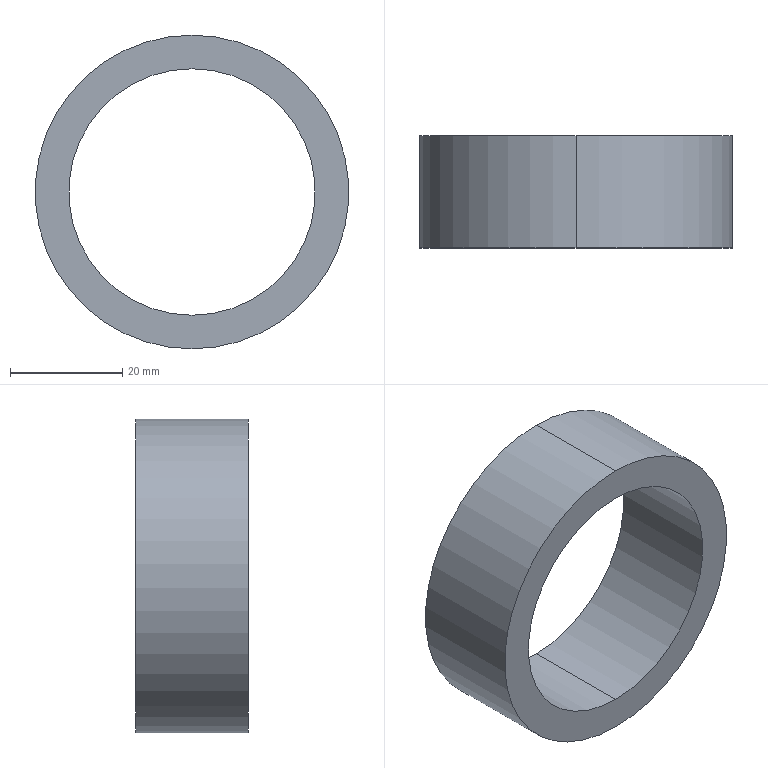Part | STEP file | outer coil2 | 1 solid | 6 faces | box 56 x 20 x 56 mm | volume 18850 mm3 | cylinder 4 | plane 2 | commonest cylinder face diameters 44 x2 56 x2
STEP:
#1=CARTESIAN_POINT('',(0.,-10.,28.));
#2=VERTEX_POINT('',#1);
#3=CARTESIAN_POINT('',(0.,-10.,-28.));
#4=VERTEX_POINT('',#3);
#5=CARTESIAN_POINT('',(0.,-10.,0.));
#6=DIRECTION('',(0.,1.,0.));
#7=DIRECTION('',(0.,0.,1.));
#8=AXIS2_PLACEMENT_3D('',#5,#6,#7);
#9=CIRCLE('',#8,28.);
#10=EDGE_CURVE('',#2,#4,#9,.T.);
#11=ORIENTED_EDGE('',*,*,#10,.T.);
#12=CARTESIAN_POINT('',(0.,10.,-28.));
#13=VERTEX_POINT('',#12);
#14=CARTESIAN_POINT('',(0.,52.348,-28.));
#15=DIRECTION('',(0.,1.,0.));
#16=VECTOR('',#15,1000.);
#17=LINE('',#14,#16);
#18=EDGE_CURVE('',#4,#13,#17,.T.);
#19=ORIENTED_EDGE('',*,*,#18,.T.);
#20=CARTESIAN_POINT('',(0.,10.,28.));
#21=VERTEX_POINT('',#20);
#22=CARTESIAN_POINT('',(0.,10.,0.));
#23=DIRECTION('',(0.,1.,0.));
#24=DIRECTION('',(0.,0.,1.));
#25=AXIS2_PLACEMENT_3D('',#22,#23,#24);
#26=CIRCLE('',#25,28.);
#27=EDGE_CURVE('',#21,#13,#26,.T.);
#28=ORIENTED_EDGE('',*,*,#27,.F.);
#29=CARTESIAN_POINT('',(0.,52.348,28.));
#30=DIRECTION('',(0.,1.,0.));
#31=VECTOR('',#30,1000.);
#32=LINE('',#29,#31);
#33=EDGE_CURVE('',#2,#21,#32,.T.);
#34=ORIENTED_EDGE('',*,*,#33,.F.);
#35=EDGE_LOOP('',(#11,#19,#28,#34));
#36=FACE_OUTER_BOUND('',#35,.T.);
#37=CARTESIAN_POINT('',(0.,52.348,0.));
#38=DIRECTION('',(0.,1.,0.));
#39=DIRECTION('',(0.,0.,1.));
#40=AXIS2_PLACEMENT_3D('',#37,#38,#39);
#41=CYLINDRICAL_SURFACE('',#40,28.);
#42=ADVANCED_FACE('',(#36),#41,.T.);
#43=CARTESIAN_POINT('',(0.,-10.,-22.));
#44=VERTEX_POINT('',#43);
#45=CARTESIAN_POINT('',(0.,-10.,22.));
#46=VERTEX_POINT('',#45);
#47=CARTESIAN_POINT('',(0.,-10.,0.));
#48=DIRECTION('',(0.,1.,0.));
#49=DIRECTION('',(0.,0.,1.));
#50=AXIS2_PLACEMENT_3D('',#47,#48,#49);
#51=CIRCLE('',#50,22.);
#52=EDGE_CURVE('',#44,#46,#51,.T.);
#53=ORIENTED_EDGE('',*,*,#52,.F.);
#54=CARTESIAN_POINT('',(0.,10.,-22.));
#55=VERTEX_POINT('',#54);
#56=CARTESIAN_POINT('',(0.,52.348,-22.));
#57=DIRECTION('',(0.,1.,0.));
#58=VECTOR('',#57,1000.);
#59=LINE('',#56,#58);
#60=EDGE_CURVE('',#44,#55,#59,.T.);
#61=ORIENTED_EDGE('',*,*,#60,.T.);
#62=CARTESIAN_POINT('',(0.,10.,22.));
#63=VERTEX_POINT('',#62);
#64=CARTESIAN_POINT('',(0.,10.,0.));
#65=DIRECTION('',(0.,1.,0.));
#66=DIRECTION('',(0.,0.,1.));
#67=AXIS2_PLACEMENT_3D('',#64,#65,#66);
#68=CIRCLE('',#67,22.);
#69=EDGE_CURVE('',#55,#63,#68,.T.);
#70=ORIENTED_EDGE('',*,*,#69,.T.);
#71=CARTESIAN_POINT('',(0.,52.348,22.));
#72=DIRECTION('',(0.,1.,0.));
#73=VECTOR('',#72,1000.);
#74=LINE('',#71,#73);
#75=EDGE_CURVE('',#46,#63,#74,.T.);
#76=ORIENTED_EDGE('',*,*,#75,.F.);
#77=EDGE_LOOP('',(#53,#61,#70,#76));
#78=FACE_OUTER_BOUND('',#77,.T.);
#79=CARTESIAN_POINT('',(0.,52.348,0.));
#80=DIRECTION('',(0.,1.,0.));
#81=DIRECTION('',(0.,0.,1.));
#82=AXIS2_PLACEMENT_3D('',#79,#80,#81);
#83=CYLINDRICAL_SURFACE('',#82,22.);
#84=ADVANCED_FACE('',(#78),#83,.F.);
#85=ORIENTED_EDGE('',*,*,#60,.F.);
#86=CARTESIAN_POINT('',(0.,-10.,0.));
#87=DIRECTION('',(0.,1.,0.));
#88=DIRECTION('',(0.,0.,1.));
#89=AXIS2_PLACEMENT_3D('',#86,#87,#88);
#90=CIRCLE('',#89,22.);
#91=EDGE_CURVE('',#46,#44,#90,.T.);
#92=ORIENTED_EDGE('',*,*,#91,.F.);
#93=ORIENTED_EDGE('',*,*,#75,.T.);
#94=CARTESIAN_POINT('',(0.,10.,0.));
#95=DIRECTION('',(0.,1.,0.));
#96=DIRECTION('',(0.,0.,1.));
#97=AXIS2_PLACEMENT_3D('',#94,#95,#96);
#98=CIRCLE('',#97,22.);
#99=EDGE_CURVE('',#63,#55,#98,.T.);
#100=ORIENTED_EDGE('',*,*,#99,.T.);
#101=EDGE_LOOP('',(#85,#92,#93,#100));
#102=FACE_OUTER_BOUND('',#101,.T.);
#103=CARTESIAN_POINT('',(0.,52.348,0.));
#104=DIRECTION('',(0.,1.,0.));
#105=DIRECTION('',(0.,0.,1.));
#106=AXIS2_PLACEMENT_3D('',#103,#104,#105);
#107=CYLINDRICAL_SURFACE('',#106,22.);
#108=ADVANCED_FACE('',(#102),#107,.F.);
#109=ORIENTED_EDGE('',*,*,#27,.T.);
#110=CARTESIAN_POINT('',(0.,10.,0.));
#111=DIRECTION('',(0.,1.,0.));
#112=DIRECTION('',(0.,0.,1.));
#113=AXIS2_PLACEMENT_3D('',#110,#111,#112);
#114=CIRCLE('',#113,28.);
#115=EDGE_CURVE('',#13,#21,#114,.T.);
#116=ORIENTED_EDGE('',*,*,#115,.T.);
#117=EDGE_LOOP('',(#109,#116));
#118=FACE_OUTER_BOUND('',#117,.T.);
#119=ORIENTED_EDGE('',*,*,#99,.F.);
#120=ORIENTED_EDGE('',*,*,#69,.F.);
#121=EDGE_LOOP('',(#119,#120));
#122=FACE_BOUND('',#121,.T.);
#123=CARTESIAN_POINT('',(-28.,10.,0.));
#124=DIRECTION('',(0.,1.,0.));
#125=DIRECTION('',(0.,0.,1.));
#126=AXIS2_PLACEMENT_3D('',#123,#124,#125);
#127=PLANE('',#126);
#128=ADVANCED_FACE('',(#118,#122),#127,.T.);
#129=ORIENTED_EDGE('',*,*,#18,.F.);
#130=CARTESIAN_POINT('',(0.,-10.,0.));
#131=DIRECTION('',(0.,1.,0.));
#132=DIRECTION('',(0.,0.,1.));
#133=AXIS2_PLACEMENT_3D('',#130,#131,#132);
#134=CIRCLE('',#133,28.);
#135=EDGE_CURVE('',#4,#2,#134,.T.);
#136=ORIENTED_EDGE('',*,*,#135,.T.);
#137=ORIENTED_EDGE('',*,*,#33,.T.);
#138=ORIENTED_EDGE('',*,*,#115,.F.);
#139=EDGE_LOOP('',(#129,#136,#137,#138));
#140=FACE_OUTER_BOUND('',#139,.T.);
#141=CARTESIAN_POINT('',(0.,52.348,0.));
#142=DIRECTION('',(0.,1.,0.));
#143=DIRECTION('',(0.,0.,1.));
#144=AXIS2_PLACEMENT_3D('',#141,#142,#143);
#145=CYLINDRICAL_SURFACE('',#144,28.);
#146=ADVANCED_FACE('',(#140),#145,.T.);
#147=ORIENTED_EDGE('',*,*,#91,.T.);
#148=ORIENTED_EDGE('',*,*,#52,.T.);
#149=EDGE_LOOP('',(#147,#148));
#150=FACE_BOUND('',#149,.T.);
#151=ORIENTED_EDGE('',*,*,#10,.F.);
#152=ORIENTED_EDGE('',*,*,#135,.F.);
#153=EDGE_LOOP('',(#151,#152));
#154=FACE_OUTER_BOUND('',#153,.T.);
#155=CARTESIAN_POINT('',(-28.,-10.,0.));
#156=DIRECTION('',(0.,-1.,0.));
#157=DIRECTION('',(0.,0.,-1.));
#158=AXIS2_PLACEMENT_3D('',#155,#156,#157);
#159=PLANE('',#158);
#160=ADVANCED_FACE('',(#150,#154),#159,.T.);
#161=CLOSED_SHELL('',(#42,#84,#108,#128,#146,#160));
#162=MANIFOLD_SOLID_BREP('',#161);
#163=CARTESIAN_POINT('',(0.,0.,0.));
#164=DIRECTION('',(0.,0.,1.));
#165=DIRECTION('',(1.,0.,0.));
#166=AXIS2_PLACEMENT_3D('',#163,#164,#165);
#167=(LENGTH_UNIT()NAMED_UNIT(*)SI_UNIT(.MILLI.,.METRE.));
#168=UNCERTAINTY_MEASURE_WITH_UNIT(LENGTH_MEASURE(0.00001),#167,'','');
#169=(NAMED_UNIT(*)PLANE_ANGLE_UNIT()SI_UNIT($,.RADIAN.));
#170=(NAMED_UNIT(*)SI_UNIT($,.STERADIAN.)SOLID_ANGLE_UNIT());
#171=(GEOMETRIC_REPRESENTATION_CONTEXT(3)GLOBAL_UNCERTAINTY_ASSIGNED_CONTEXT((#168))GLOBAL_UNIT_ASSIGNED_CONTEXT((#167,#169,#170))REPRESENTATION_CONTEXT('',''));
#172=ADVANCED_BREP_SHAPE_REPRESENTATION('',(#162,#166),#171);